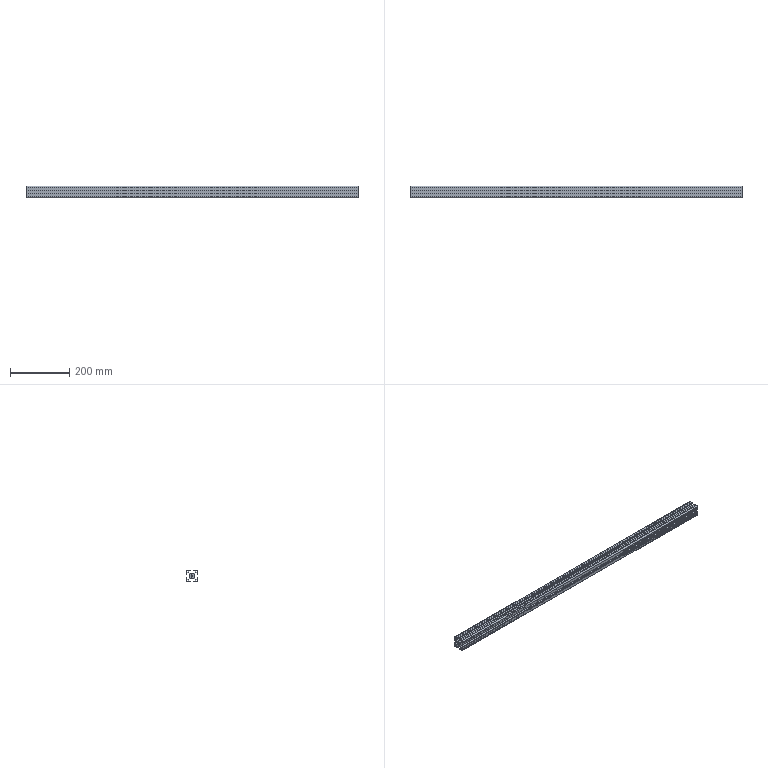Part | 1 solid | 104 faces | box 1125 x 40 x 40 mm | volume 648614 mm3 | plane 94 | cylinder 10 | commonest cylinder face diameters 5 x4 9 x4 6.8 x2